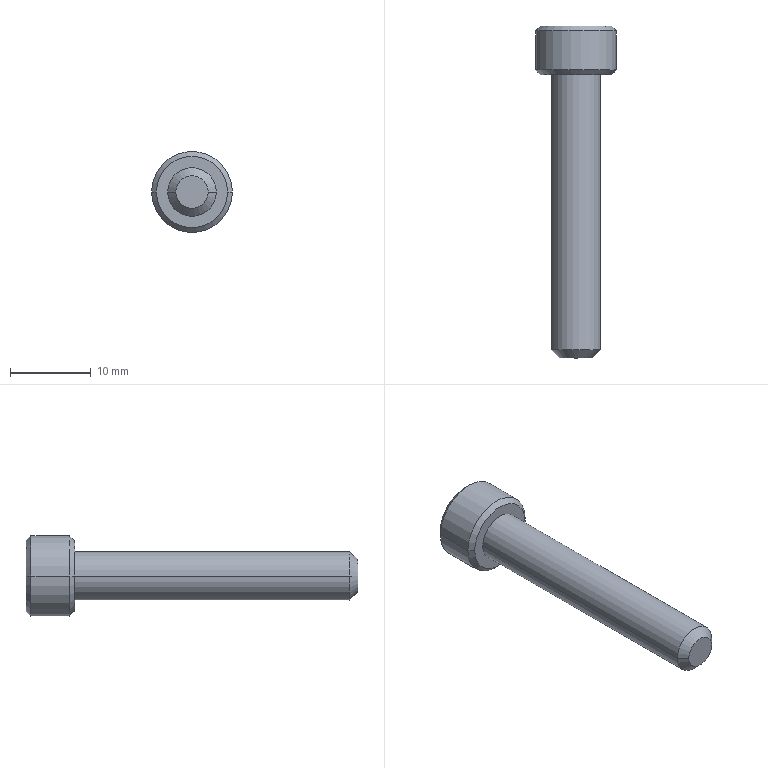Part | STEP file | BB62-M6-35L-3 | 1 solid | 27 faces | box 10 x 41 x 10 mm | volume 1364 mm3 | plane 15 | cone 8 | cylinder 4 | commonest cylinder face diameters 6 x2 10 x2
STEP:
#1=CARTESIAN_POINT('',(0.,1.349,0.));
#2=VERTEX_POINT('',#1);
#3=CARTESIAN_POINT('',(2.86,3.,0.));
#4=VERTEX_POINT('',#3);
#5=CARTESIAN_POINT('',(0.,1.349,0.));
#6=DIRECTION('',(0.866,0.5,0.));
#7=VECTOR('',#6,1000.);
#8=LINE('',#5,#7);
#9=EDGE_CURVE('',#2,#4,#8,.T.);
#10=ORIENTED_EDGE('',*,*,#9,.F.);
#11=CARTESIAN_POINT('',(-2.86,3.,0.));
#12=VERTEX_POINT('',#11);
#13=CARTESIAN_POINT('',(0.,1.349,0.));
#14=DIRECTION('',(-0.866,0.5,0.));
#15=VECTOR('',#14,1000.);
#16=LINE('',#13,#15);
#17=EDGE_CURVE('',#2,#12,#16,.T.);
#18=ORIENTED_EDGE('',*,*,#17,.T.);
#19=CARTESIAN_POINT('',(-2.477,3.,1.43));
#20=VERTEX_POINT('',#19);
#21=CARTESIAN_POINT('',(0.,3.,0.));
#22=DIRECTION('',(0.,-1.,0.));
#23=DIRECTION('',(-1.,0.,0.));
#24=AXIS2_PLACEMENT_3D('',#21,#22,#23);
#25=CIRCLE('',#24,2.86);
#26=EDGE_CURVE('',#20,#12,#25,.T.);
#27=ORIENTED_EDGE('',*,*,#26,.F.);
#28=CARTESIAN_POINT('',(0.,3.,2.86));
#29=VERTEX_POINT('',#28);
#30=CARTESIAN_POINT('',(0.,3.,0.));
#31=DIRECTION('',(0.,-1.,0.));
#32=DIRECTION('',(-1.,0.,0.));
#33=AXIS2_PLACEMENT_3D('',#30,#31,#32);
#34=CIRCLE('',#33,2.86);
#35=EDGE_CURVE('',#29,#20,#34,.T.);
#36=ORIENTED_EDGE('',*,*,#35,.F.);
#37=CARTESIAN_POINT('',(2.477,3.,1.43));
#38=VERTEX_POINT('',#37);
#39=CARTESIAN_POINT('',(0.,3.,0.));
#40=DIRECTION('',(0.,-1.,0.));
#41=DIRECTION('',(-1.,0.,0.));
#42=AXIS2_PLACEMENT_3D('',#39,#40,#41);
#43=CIRCLE('',#42,2.86);
#44=EDGE_CURVE('',#38,#29,#43,.T.);
#45=ORIENTED_EDGE('',*,*,#44,.F.);
#46=CARTESIAN_POINT('',(0.,3.,0.));
#47=DIRECTION('',(0.,-1.,0.));
#48=DIRECTION('',(-1.,0.,0.));
#49=AXIS2_PLACEMENT_3D('',#46,#47,#48);
#50=CIRCLE('',#49,2.86);
#51=EDGE_CURVE('',#4,#38,#50,.T.);
#52=ORIENTED_EDGE('',*,*,#51,.F.);
#53=EDGE_LOOP('',(#10,#18,#27,#36,#45,#52));
#54=FACE_OUTER_BOUND('',#53,.T.);
#55=CARTESIAN_POINT('',(0.,1001.349,0.));
#56=DIRECTION('',(0.,1.,0.));
#57=DIRECTION('',(1.,0.,0.));
#58=AXIS2_PLACEMENT_3D('',#55,#56,#57);
#59=CONICAL_SURFACE('',#58,1732.051,1.047);
#60=ADVANCED_FACE('',(#54),#59,.F.);
#61=CARTESIAN_POINT('',(2.,-35.,0.));
#62=VERTEX_POINT('',#61);
#63=CARTESIAN_POINT('',(-2.,-35.,0.));
#64=VERTEX_POINT('',#63);
#65=CARTESIAN_POINT('',(0.,-35.,0.));
#66=DIRECTION('',(0.,1.,0.));
#67=DIRECTION('',(1.,0.,0.));
#68=AXIS2_PLACEMENT_3D('',#65,#66,#67);
#69=CIRCLE('',#68,2.);
#70=EDGE_CURVE('',#62,#64,#69,.T.);
#71=ORIENTED_EDGE('',*,*,#70,.T.);
#72=CARTESIAN_POINT('',(-3.,-34.,0.));
#73=VERTEX_POINT('',#72);
#74=CARTESIAN_POINT('',(-2.,-35.,0.));
#75=DIRECTION('',(-0.7071,0.7071,0.));
#76=VECTOR('',#75,1000.);
#77=LINE('',#74,#76);
#78=EDGE_CURVE('',#64,#73,#77,.T.);
#79=ORIENTED_EDGE('',*,*,#78,.T.);
#80=CARTESIAN_POINT('',(3.,-34.,0.));
#81=VERTEX_POINT('',#80);
#82=CARTESIAN_POINT('',(0.,-34.,0.));
#83=DIRECTION('',(0.,-1.,0.));
#84=DIRECTION('',(-1.,0.,0.));
#85=AXIS2_PLACEMENT_3D('',#82,#83,#84);
#86=CIRCLE('',#85,3.);
#87=EDGE_CURVE('',#73,#81,#86,.T.);
#88=ORIENTED_EDGE('',*,*,#87,.T.);
#89=CARTESIAN_POINT('',(2.,-35.,0.));
#90=DIRECTION('',(0.7071,0.7071,0.));
#91=VECTOR('',#90,1000.);
#92=LINE('',#89,#91);
#93=EDGE_CURVE('',#62,#81,#92,.T.);
#94=ORIENTED_EDGE('',*,*,#93,.F.);
#95=EDGE_LOOP('',(#71,#79,#88,#94));
#96=FACE_OUTER_BOUND('',#95,.T.);
#97=CARTESIAN_POINT('',(0.,-35.,0.));
#98=DIRECTION('',(0.,1.,0.));
#99=DIRECTION('',(1.,0.,0.));
#100=AXIS2_PLACEMENT_3D('',#97,#98,#99);
#101=CONICAL_SURFACE('',#100,2.,0.7854);
#102=ADVANCED_FACE('',(#96),#101,.T.);
#103=ORIENTED_EDGE('',*,*,#87,.F.);
#104=CARTESIAN_POINT('',(-3.,0.,0.));
#105=VERTEX_POINT('',#104);
#106=CARTESIAN_POINT('',(-3.,-34.,0.));
#107=DIRECTION('',(0.,1.,0.));
#108=VECTOR('',#107,1000.);
#109=LINE('',#106,#108);
#110=EDGE_CURVE('',#73,#105,#109,.T.);
#111=ORIENTED_EDGE('',*,*,#110,.T.);
#112=CARTESIAN_POINT('',(3.,0.,0.));
#113=VERTEX_POINT('',#112);
#114=CARTESIAN_POINT('',(0.,0.,0.));
#115=DIRECTION('',(0.,-1.,0.));
#116=DIRECTION('',(-1.,0.,0.));
#117=AXIS2_PLACEMENT_3D('',#114,#115,#116);
#118=CIRCLE('',#117,3.);
#119=EDGE_CURVE('',#105,#113,#118,.T.);
#120=ORIENTED_EDGE('',*,*,#119,.T.);
#121=CARTESIAN_POINT('',(3.,-34.,0.));
#122=DIRECTION('',(0.,1.,0.));
#123=VECTOR('',#122,1000.);
#124=LINE('',#121,#123);
#125=EDGE_CURVE('',#81,#113,#124,.T.);
#126=ORIENTED_EDGE('',*,*,#125,.F.);
#127=EDGE_LOOP('',(#103,#111,#120,#126));
#128=FACE_OUTER_BOUND('',#127,.T.);
#129=CARTESIAN_POINT('',(0.,-34.,0.));
#130=DIRECTION('',(0.,1.,0.));
#131=DIRECTION('',(1.,0.,0.));
#132=AXIS2_PLACEMENT_3D('',#129,#130,#131);
#133=CYLINDRICAL_SURFACE('',#132,3.);
#134=ADVANCED_FACE('',(#128),#133,.T.);
#135=CARTESIAN_POINT('',(-4.4,6.,0.));
#136=VERTEX_POINT('',#135);
#137=CARTESIAN_POINT('',(4.4,6.,0.));
#138=VERTEX_POINT('',#137);
#139=CARTESIAN_POINT('',(0.,6.,0.));
#140=DIRECTION('',(0.,-1.,0.));
#141=DIRECTION('',(-1.,0.,0.));
#142=AXIS2_PLACEMENT_3D('',#139,#140,#141);
#143=CIRCLE('',#142,4.4);
#144=EDGE_CURVE('',#136,#138,#143,.T.);
#145=ORIENTED_EDGE('',*,*,#144,.T.);
#146=CARTESIAN_POINT('',(5.,5.4,0.));
#147=VERTEX_POINT('',#146);
#148=CARTESIAN_POINT('',(5.,5.4,0.));
#149=DIRECTION('',(0.7071,-0.7071,0.));
#150=VECTOR('',#149,1000.);
#151=LINE('',#148,#150);
#152=EDGE_CURVE('',#138,#147,#151,.T.);
#153=ORIENTED_EDGE('',*,*,#152,.T.);
#154=CARTESIAN_POINT('',(-5.,5.4,0.));
#155=VERTEX_POINT('',#154);
#156=CARTESIAN_POINT('',(0.,5.4,0.));
#157=DIRECTION('',(0.,-1.,0.));
#158=DIRECTION('',(-1.,0.,0.));
#159=AXIS2_PLACEMENT_3D('',#156,#157,#158);
#160=CIRCLE('',#159,5.);
#161=EDGE_CURVE('',#155,#147,#160,.T.);
#162=ORIENTED_EDGE('',*,*,#161,.F.);
#163=CARTESIAN_POINT('',(-5.,5.4,0.));
#164=DIRECTION('',(-0.7071,-0.7071,0.));
#165=VECTOR('',#164,1000.);
#166=LINE('',#163,#165);
#167=EDGE_CURVE('',#136,#155,#166,.T.);
#168=ORIENTED_EDGE('',*,*,#167,.F.);
#169=EDGE_LOOP('',(#145,#153,#162,#168));
#170=FACE_OUTER_BOUND('',#169,.T.);
#171=CARTESIAN_POINT('',(0.,5.4,0.));
#172=DIRECTION('',(0.,-1.,0.));
#173=DIRECTION('',(-1.,0.,0.));
#174=AXIS2_PLACEMENT_3D('',#171,#172,#173);
#175=CONICAL_SURFACE('',#174,5.,0.7854);
#176=ADVANCED_FACE('',(#170),#175,.T.);
#177=ORIENTED_EDGE('',*,*,#161,.T.);
#178=CARTESIAN_POINT('',(5.,0.6,0.));
#179=VERTEX_POINT('',#178);
#180=CARTESIAN_POINT('',(5.,1.62,0.));
#181=DIRECTION('',(0.,-1.,0.));
#182=VECTOR('',#181,1000.);
#183=LINE('',#180,#182);
#184=EDGE_CURVE('',#147,#179,#183,.T.);
#185=ORIENTED_EDGE('',*,*,#184,.T.);
#186=CARTESIAN_POINT('',(-5.,0.6,0.));
#187=VERTEX_POINT('',#186);
#188=CARTESIAN_POINT('',(0.,0.6,0.));
#189=DIRECTION('',(0.,-1.,0.));
#190=DIRECTION('',(-1.,0.,0.));
#191=AXIS2_PLACEMENT_3D('',#188,#189,#190);
#192=CIRCLE('',#191,5.);
#193=EDGE_CURVE('',#187,#179,#192,.T.);
#194=ORIENTED_EDGE('',*,*,#193,.F.);
#195=CARTESIAN_POINT('',(-5.,1.62,0.));
#196=DIRECTION('',(0.,-1.,0.));
#197=VECTOR('',#196,1000.);
#198=LINE('',#195,#197);
#199=EDGE_CURVE('',#155,#187,#198,.T.);
#200=ORIENTED_EDGE('',*,*,#199,.F.);
#201=EDGE_LOOP('',(#177,#185,#194,#200));
#202=FACE_OUTER_BOUND('',#201,.T.);
#203=CARTESIAN_POINT('',(0.,1.62,0.));
#204=DIRECTION('',(0.,-1.,0.));
#205=DIRECTION('',(-1.,0.,0.));
#206=AXIS2_PLACEMENT_3D('',#203,#204,#205);
#207=CYLINDRICAL_SURFACE('',#206,5.);
#208=ADVANCED_FACE('',(#202),#207,.T.);
#209=CARTESIAN_POINT('',(-4.4,0.,0.));
#210=VERTEX_POINT('',#209);
#211=CARTESIAN_POINT('',(4.4,0.,0.));
#212=VERTEX_POINT('',#211);
#213=CARTESIAN_POINT('',(0.,0.,0.));
#214=DIRECTION('',(0.,-1.,0.));
#215=DIRECTION('',(-1.,0.,0.));
#216=AXIS2_PLACEMENT_3D('',#213,#214,#215);
#217=CIRCLE('',#216,4.4);
#218=EDGE_CURVE('',#210,#212,#217,.T.);
#219=ORIENTED_EDGE('',*,*,#218,.F.);
#220=CARTESIAN_POINT('',(-4.4,0.,0.));
#221=DIRECTION('',(-0.7071,0.7071,0.));
#222=VECTOR('',#221,1000.);
#223=LINE('',#220,#222);
#224=EDGE_CURVE('',#210,#187,#223,.T.);
#225=ORIENTED_EDGE('',*,*,#224,.T.);
#226=ORIENTED_EDGE('',*,*,#193,.T.);
#227=CARTESIAN_POINT('',(4.4,0.,0.));
#228=DIRECTION('',(0.7071,0.7071,0.));
#229=VECTOR('',#228,1000.);
#230=LINE('',#227,#229);
#231=EDGE_CURVE('',#212,#179,#230,.T.);
#232=ORIENTED_EDGE('',*,*,#231,.F.);
#233=EDGE_LOOP('',(#219,#225,#226,#232));
#234=FACE_OUTER_BOUND('',#233,.T.);
#235=CARTESIAN_POINT('',(0.,0.,0.));
#236=DIRECTION('',(0.,1.,0.));
#237=DIRECTION('',(1.,0.,0.));
#238=AXIS2_PLACEMENT_3D('',#235,#236,#237);
#239=CONICAL_SURFACE('',#238,4.4,0.7854);
#240=ADVANCED_FACE('',(#234),#239,.T.);
#241=ORIENTED_EDGE('',*,*,#144,.F.);
#242=CARTESIAN_POINT('',(0.,6.,0.));
#243=DIRECTION('',(0.,-1.,0.));
#244=DIRECTION('',(-1.,0.,0.));
#245=AXIS2_PLACEMENT_3D('',#242,#243,#244);
#246=CIRCLE('',#245,4.4);
#247=EDGE_CURVE('',#138,#136,#246,.T.);
#248=ORIENTED_EDGE('',*,*,#247,.F.);
#249=EDGE_LOOP('',(#241,#248));
#250=FACE_OUTER_BOUND('',#249,.T.);
#251=CARTESIAN_POINT('',(0.,6.,-2.86));
#252=VERTEX_POINT('',#251);
#253=CARTESIAN_POINT('',(-2.477,6.,-1.43));
#254=VERTEX_POINT('',#253);
#255=CARTESIAN_POINT('',(0.,6.,-2.86));
#256=DIRECTION('',(-0.866,0.,0.5));
#257=VECTOR('',#256,1000.);
#258=LINE('',#255,#257);
#259=EDGE_CURVE('',#252,#254,#258,.T.);
#260=ORIENTED_EDGE('',*,*,#259,.F.);
#261=CARTESIAN_POINT('',(2.477,6.,-1.43));
#262=VERTEX_POINT('',#261);
#263=CARTESIAN_POINT('',(2.477,6.,-1.43));
#264=DIRECTION('',(-0.866,0.,-0.5));
#265=VECTOR('',#264,1000.);
#266=LINE('',#263,#265);
#267=EDGE_CURVE('',#262,#252,#266,.T.);
#268=ORIENTED_EDGE('',*,*,#267,.F.);
#269=CARTESIAN_POINT('',(2.477,6.,1.43));
#270=VERTEX_POINT('',#269);
#271=CARTESIAN_POINT('',(2.477,6.,1.43));
#272=DIRECTION('',(0.,0.,-1.));
#273=VECTOR('',#272,1000.);
#274=LINE('',#271,#273);
#275=EDGE_CURVE('',#270,#262,#274,.T.);
#276=ORIENTED_EDGE('',*,*,#275,.F.);
#277=CARTESIAN_POINT('',(0.,6.,2.86));
#278=VERTEX_POINT('',#277);
#279=CARTESIAN_POINT('',(0.,6.,2.86));
#280=DIRECTION('',(0.866,0.,-0.5));
#281=VECTOR('',#280,1000.);
#282=LINE('',#279,#281);
#283=EDGE_CURVE('',#278,#270,#282,.T.);
#284=ORIENTED_EDGE('',*,*,#283,.F.);
#285=CARTESIAN_POINT('',(-2.477,6.,1.43));
#286=VERTEX_POINT('',#285);
#287=CARTESIAN_POINT('',(-2.477,6.,1.43));
#288=DIRECTION('',(0.866,0.,0.5));
#289=VECTOR('',#288,1000.);
#290=LINE('',#287,#289);
#291=EDGE_CURVE('',#286,#278,#290,.T.);
#292=ORIENTED_EDGE('',*,*,#291,.F.);
#293=CARTESIAN_POINT('',(-2.477,6.,-1.43));
#294=DIRECTION('',(0.,0.,1.));
#295=VECTOR('',#294,1000.);
#296=LINE('',#293,#295);
#297=EDGE_CURVE('',#254,#286,#296,.T.);
#298=ORIENTED_EDGE('',*,*,#297,.F.);
#299=EDGE_LOOP('',(#260,#268,#276,#284,#292,#298));
#300=FACE_BOUND('',#299,.T.);
#301=CARTESIAN_POINT('',(4.4,6.,0.));
#302=DIRECTION('',(0.,1.,0.));
#303=DIRECTION('',(1.,0.,0.));
#304=AXIS2_PLACEMENT_3D('',#301,#302,#303);
#305=PLANE('',#304);
#306=ADVANCED_FACE('',(#250,#300),#305,.T.);
#307=CARTESIAN_POINT('',(0.,0.,0.));
#308=DIRECTION('',(0.,-1.,0.));
#309=DIRECTION('',(-1.,0.,0.));
#310=AXIS2_PLACEMENT_3D('',#307,#308,#309);
#311=CIRCLE('',#310,3.);
#312=EDGE_CURVE('',#113,#105,#311,.T.);
#313=ORIENTED_EDGE('',*,*,#312,.F.);
#314=ORIENTED_EDGE('',*,*,#119,.F.);
#315=EDGE_LOOP('',(#313,#314));
#316=FACE_BOUND('',#315,.T.);
#317=CARTESIAN_POINT('',(0.,0.,0.));
#318=DIRECTION('',(0.,-1.,0.));
#319=DIRECTION('',(-1.,0.,0.));
#320=AXIS2_PLACEMENT_3D('',#317,#318,#319);
#321=CIRCLE('',#320,4.4);
#322=EDGE_CURVE('',#212,#210,#321,.T.);
#323=ORIENTED_EDGE('',*,*,#322,.T.);
#324=ORIENTED_EDGE('',*,*,#218,.T.);
#325=EDGE_LOOP('',(#323,#324));
#326=FACE_OUTER_BOUND('',#325,.T.);
#327=CARTESIAN_POINT('',(0.,0.,0.));
#328=DIRECTION('',(0.,-1.,0.));
#329=DIRECTION('',(-1.,0.,0.));
#330=AXIS2_PLACEMENT_3D('',#327,#328,#329);
#331=PLANE('',#330);
#332=ADVANCED_FACE('',(#316,#326),#331,.T.);
#333=ORIENTED_EDGE('',*,*,#224,.F.);
#334=ORIENTED_EDGE('',*,*,#322,.F.);
#335=ORIENTED_EDGE('',*,*,#231,.T.);
#336=CARTESIAN_POINT('',(0.,0.6,0.));
#337=DIRECTION('',(0.,-1.,0.));
#338=DIRECTION('',(-1.,0.,0.));
#339=AXIS2_PLACEMENT_3D('',#336,#337,#338);
#340=CIRCLE('',#339,5.);
#341=EDGE_CURVE('',#179,#187,#340,.T.);
#342=ORIENTED_EDGE('',*,*,#341,.T.);
#343=EDGE_LOOP('',(#333,#334,#335,#342));
#344=FACE_OUTER_BOUND('',#343,.T.);
#345=CARTESIAN_POINT('',(0.,0.,0.));
#346=DIRECTION('',(0.,1.,0.));
#347=DIRECTION('',(1.,0.,0.));
#348=AXIS2_PLACEMENT_3D('',#345,#346,#347);
#349=CONICAL_SURFACE('',#348,4.4,0.7854);
#350=ADVANCED_FACE('',(#344),#349,.T.);
#351=ORIENTED_EDGE('',*,*,#184,.F.);
#352=CARTESIAN_POINT('',(0.,5.4,0.));
#353=DIRECTION('',(0.,-1.,0.));
#354=DIRECTION('',(-1.,0.,0.));
#355=AXIS2_PLACEMENT_3D('',#352,#353,#354);
#356=CIRCLE('',#355,5.);
#357=EDGE_CURVE('',#147,#155,#356,.T.);
#358=ORIENTED_EDGE('',*,*,#357,.T.);
#359=ORIENTED_EDGE('',*,*,#199,.T.);
#360=ORIENTED_EDGE('',*,*,#341,.F.);
#361=EDGE_LOOP('',(#351,#358,#359,#360));
#362=FACE_OUTER_BOUND('',#361,.T.);
#363=CARTESIAN_POINT('',(0.,1.62,0.));
#364=DIRECTION('',(0.,-1.,0.));
#365=DIRECTION('',(-1.,0.,0.));
#366=AXIS2_PLACEMENT_3D('',#363,#364,#365);
#367=CYLINDRICAL_SURFACE('',#366,5.);
#368=ADVANCED_FACE('',(#362),#367,.T.);
#369=ORIENTED_EDGE('',*,*,#152,.F.);
#370=ORIENTED_EDGE('',*,*,#247,.T.);
#371=ORIENTED_EDGE('',*,*,#167,.T.);
#372=ORIENTED_EDGE('',*,*,#357,.F.);
#373=EDGE_LOOP('',(#369,#370,#371,#372));
#374=FACE_OUTER_BOUND('',#373,.T.);
#375=CARTESIAN_POINT('',(0.,5.4,0.));
#376=DIRECTION('',(0.,-1.,0.));
#377=DIRECTION('',(-1.,0.,0.));
#378=AXIS2_PLACEMENT_3D('',#375,#376,#377);
#379=CONICAL_SURFACE('',#378,5.,0.7854);
#380=ADVANCED_FACE('',(#374),#379,.T.);
#381=ORIENTED_EDGE('',*,*,#110,.F.);
#382=CARTESIAN_POINT('',(0.,-34.,0.));
#383=DIRECTION('',(0.,-1.,0.));
#384=DIRECTION('',(-1.,0.,0.));
#385=AXIS2_PLACEMENT_3D('',#382,#383,#384);
#386=CIRCLE('',#385,3.);
#387=EDGE_CURVE('',#81,#73,#386,.T.);
#388=ORIENTED_EDGE('',*,*,#387,.F.);
#389=ORIENTED_EDGE('',*,*,#125,.T.);
#390=ORIENTED_EDGE('',*,*,#312,.T.);
#391=EDGE_LOOP('',(#381,#388,#389,#390));
#392=FACE_OUTER_BOUND('',#391,.T.);
#393=CARTESIAN_POINT('',(0.,-34.,0.));
#394=DIRECTION('',(0.,1.,0.));
#395=DIRECTION('',(1.,0.,0.));
#396=AXIS2_PLACEMENT_3D('',#393,#394,#395);
#397=CYLINDRICAL_SURFACE('',#396,3.);
#398=ADVANCED_FACE('',(#392),#397,.T.);
#399=ORIENTED_EDGE('',*,*,#70,.F.);
#400=CARTESIAN_POINT('',(0.,-35.,0.));
#401=DIRECTION('',(0.,1.,0.));
#402=DIRECTION('',(1.,0.,0.));
#403=AXIS2_PLACEMENT_3D('',#400,#401,#402);
#404=CIRCLE('',#403,2.);
#405=EDGE_CURVE('',#64,#62,#404,.T.);
#406=ORIENTED_EDGE('',*,*,#405,.F.);
#407=EDGE_LOOP('',(#399,#406));
#408=FACE_OUTER_BOUND('',#407,.T.);
#409=CARTESIAN_POINT('',(0.,-35.,0.));
#410=DIRECTION('',(0.,-1.,0.));
#411=DIRECTION('',(-1.,0.,0.));
#412=AXIS2_PLACEMENT_3D('',#409,#410,#411);
#413=PLANE('',#412);
#414=ADVANCED_FACE('',(#408),#413,.T.);
#415=ORIENTED_EDGE('',*,*,#78,.F.);
#416=ORIENTED_EDGE('',*,*,#405,.T.);
#417=ORIENTED_EDGE('',*,*,#93,.T.);
#418=ORIENTED_EDGE('',*,*,#387,.T.);
#419=EDGE_LOOP('',(#415,#416,#417,#418));
#420=FACE_OUTER_BOUND('',#419,.T.);
#421=CARTESIAN_POINT('',(0.,-35.,0.));
#422=DIRECTION('',(0.,1.,0.));
#423=DIRECTION('',(1.,0.,0.));
#424=AXIS2_PLACEMENT_3D('',#421,#422,#423);
#425=CONICAL_SURFACE('',#424,2.,0.7854);
#426=ADVANCED_FACE('',(#420),#425,.T.);
#427=CARTESIAN_POINT('',(2.477,3.,-1.43));
#428=VERTEX_POINT('',#427);
#429=CARTESIAN_POINT('',(0.,3.,-2.86));
#430=VERTEX_POINT('',#429);
#431=CARTESIAN_POINT('',(2.477,3.,-1.43));
#432=DIRECTION('',(-0.866,0.,-0.5));
#433=VECTOR('',#432,1000.);
#434=LINE('',#431,#433);
#435=EDGE_CURVE('',#428,#430,#434,.T.);
#436=ORIENTED_EDGE('',*,*,#435,.F.);
#437=CARTESIAN_POINT('',(2.477,6.,-1.43));
#438=DIRECTION('',(0.,-1.,0.));
#439=VECTOR('',#438,1000.);
#440=LINE('',#437,#439);
#441=EDGE_CURVE('',#262,#428,#440,.T.);
#442=ORIENTED_EDGE('',*,*,#441,.F.);
#443=ORIENTED_EDGE('',*,*,#267,.T.);
#444=CARTESIAN_POINT('',(0.,6.,-2.86));
#445=DIRECTION('',(0.,-1.,0.));
#446=VECTOR('',#445,1000.);
#447=LINE('',#444,#446);
#448=EDGE_CURVE('',#252,#430,#447,.T.);
#449=ORIENTED_EDGE('',*,*,#448,.T.);
#450=EDGE_LOOP('',(#436,#442,#443,#449));
#451=FACE_OUTER_BOUND('',#450,.T.);
#452=CARTESIAN_POINT('',(2.477,6.,-1.43));
#453=DIRECTION('',(-0.5,0.,0.866));
#454=DIRECTION('',(0.866,0.,0.5));
#455=AXIS2_PLACEMENT_3D('',#452,#453,#454);
#456=PLANE('',#455);
#457=ADVANCED_FACE('',(#451),#456,.T.);
#458=CARTESIAN_POINT('',(-2.477,3.,-1.43));
#459=VERTEX_POINT('',#458);
#460=CARTESIAN_POINT('',(0.,3.,-2.86));
#461=DIRECTION('',(-0.866,0.,0.5));
#462=VECTOR('',#461,1000.);
#463=LINE('',#460,#462);
#464=EDGE_CURVE('',#430,#459,#463,.T.);
#465=ORIENTED_EDGE('',*,*,#464,.F.);
#466=ORIENTED_EDGE('',*,*,#448,.F.);
#467=ORIENTED_EDGE('',*,*,#259,.T.);
#468=CARTESIAN_POINT('',(-2.477,6.,-1.43));
#469=DIRECTION('',(0.,-1.,0.));
#470=VECTOR('',#469,1000.);
#471=LINE('',#468,#470);
#472=EDGE_CURVE('',#254,#459,#471,.T.);
#473=ORIENTED_EDGE('',*,*,#472,.T.);
#474=EDGE_LOOP('',(#465,#466,#467,#473));
#475=FACE_OUTER_BOUND('',#474,.T.);
#476=CARTESIAN_POINT('',(0.,6.,-2.86));
#477=DIRECTION('',(0.5,0.,0.866));
#478=DIRECTION('',(0.866,0.,-0.5));
#479=AXIS2_PLACEMENT_3D('',#476,#477,#478);
#480=PLANE('',#479);
#481=ADVANCED_FACE('',(#475),#480,.T.);
#482=CARTESIAN_POINT('',(-2.477,3.,-1.43));
#483=DIRECTION('',(0.,0.,1.));
#484=VECTOR('',#483,1000.);
#485=LINE('',#482,#484);
#486=EDGE_CURVE('',#459,#20,#485,.T.);
#487=ORIENTED_EDGE('',*,*,#486,.F.);
#488=ORIENTED_EDGE('',*,*,#472,.F.);
#489=ORIENTED_EDGE('',*,*,#297,.T.);
#490=CARTESIAN_POINT('',(-2.477,6.,1.43));
#491=DIRECTION('',(0.,-1.,0.));
#492=VECTOR('',#491,1000.);
#493=LINE('',#490,#492);
#494=EDGE_CURVE('',#286,#20,#493,.T.);
#495=ORIENTED_EDGE('',*,*,#494,.T.);
#496=EDGE_LOOP('',(#487,#488,#489,#495));
#497=FACE_OUTER_BOUND('',#496,.T.);
#498=CARTESIAN_POINT('',(-2.477,6.,-1.43));
#499=DIRECTION('',(1.,0.,0.));
#500=DIRECTION('',(0.,0.,-1.));
#501=AXIS2_PLACEMENT_3D('',#498,#499,#500);
#502=PLANE('',#501);
#503=ADVANCED_FACE('',(#497),#502,.T.);
#504=CARTESIAN_POINT('',(-2.477,3.,1.43));
#505=DIRECTION('',(0.866,0.,0.5));
#506=VECTOR('',#505,1000.);
#507=LINE('',#504,#506);
#508=EDGE_CURVE('',#20,#29,#507,.T.);
#509=ORIENTED_EDGE('',*,*,#508,.F.);
#510=ORIENTED_EDGE('',*,*,#494,.F.);
#511=ORIENTED_EDGE('',*,*,#291,.T.);
#512=CARTESIAN_POINT('',(0.,6.,2.86));
#513=DIRECTION('',(0.,-1.,0.));
#514=VECTOR('',#513,1000.);
#515=LINE('',#512,#514);
#516=EDGE_CURVE('',#278,#29,#515,.T.);
#517=ORIENTED_EDGE('',*,*,#516,.T.);
#518=EDGE_LOOP('',(#509,#510,#511,#517));
#519=FACE_OUTER_BOUND('',#518,.T.);
#520=CARTESIAN_POINT('',(-2.477,6.,1.43));
#521=DIRECTION('',(0.5,0.,-0.866));
#522=DIRECTION('',(-0.866,0.,-0.5));
#523=AXIS2_PLACEMENT_3D('',#520,#521,#522);
#524=PLANE('',#523);
#525=ADVANCED_FACE('',(#519),#524,.T.);
#526=CARTESIAN_POINT('',(0.,3.,2.86));
#527=DIRECTION('',(0.866,0.,-0.5));
#528=VECTOR('',#527,1000.);
#529=LINE('',#526,#528);
#530=EDGE_CURVE('',#29,#38,#529,.T.);
#531=ORIENTED_EDGE('',*,*,#530,.F.);
#532=ORIENTED_EDGE('',*,*,#516,.F.);
#533=ORIENTED_EDGE('',*,*,#283,.T.);
#534=CARTESIAN_POINT('',(2.477,6.,1.43));
#535=DIRECTION('',(0.,-1.,0.));
#536=VECTOR('',#535,1000.);
#537=LINE('',#534,#536);
#538=EDGE_CURVE('',#270,#38,#537,.T.);
#539=ORIENTED_EDGE('',*,*,#538,.T.);
#540=EDGE_LOOP('',(#531,#532,#533,#539));
#541=FACE_OUTER_BOUND('',#540,.T.);
#542=CARTESIAN_POINT('',(0.,6.,2.86));
#543=DIRECTION('',(-0.5,0.,-0.866));
#544=DIRECTION('',(-0.866,0.,0.5));
#545=AXIS2_PLACEMENT_3D('',#542,#543,#544);
#546=PLANE('',#545);
#547=ADVANCED_FACE('',(#541),#546,.T.);
#548=CARTESIAN_POINT('',(2.477,3.,1.43));
#549=DIRECTION('',(0.,0.,-1.));
#550=VECTOR('',#549,1000.);
#551=LINE('',#548,#550);
#552=EDGE_CURVE('',#38,#428,#551,.T.);
#553=ORIENTED_EDGE('',*,*,#552,.F.);
#554=ORIENTED_EDGE('',*,*,#538,.F.);
#555=ORIENTED_EDGE('',*,*,#275,.T.);
#556=ORIENTED_EDGE('',*,*,#441,.T.);
#557=EDGE_LOOP('',(#553,#554,#555,#556));
#558=FACE_OUTER_BOUND('',#557,.T.);
#559=CARTESIAN_POINT('',(2.477,6.,1.43));
#560=DIRECTION('',(-1.,0.,0.));
#561=DIRECTION('',(0.,0.,1.));
#562=AXIS2_PLACEMENT_3D('',#559,#560,#561);
#563=PLANE('',#562);
#564=ADVANCED_FACE('',(#558),#563,.T.);
#565=ORIENTED_EDGE('',*,*,#435,.T.);
#566=CARTESIAN_POINT('',(0.,3.,0.));
#567=DIRECTION('',(0.,-1.,0.));
#568=DIRECTION('',(-1.,0.,0.));
#569=AXIS2_PLACEMENT_3D('',#566,#567,#568);
#570=CIRCLE('',#569,2.86);
#571=EDGE_CURVE('',#430,#428,#570,.T.);
#572=ORIENTED_EDGE('',*,*,#571,.T.);
#573=EDGE_LOOP('',(#565,#572));
#574=FACE_OUTER_BOUND('',#573,.T.);
#575=CARTESIAN_POINT('',(0.,3.,0.));
#576=DIRECTION('',(0.,1.,0.));
#577=DIRECTION('',(1.,0.,0.));
#578=AXIS2_PLACEMENT_3D('',#575,#576,#577);
#579=PLANE('',#578);
#580=ADVANCED_FACE('',(#574),#579,.F.);
#581=ORIENTED_EDGE('',*,*,#552,.T.);
#582=CARTESIAN_POINT('',(0.,3.,0.));
#583=DIRECTION('',(0.,-1.,0.));
#584=DIRECTION('',(-1.,0.,0.));
#585=AXIS2_PLACEMENT_3D('',#582,#583,#584);
#586=CIRCLE('',#585,2.86);
#587=EDGE_CURVE('',#428,#4,#586,.T.);
#588=ORIENTED_EDGE('',*,*,#587,.T.);
#589=ORIENTED_EDGE('',*,*,#51,.T.);
#590=EDGE_LOOP('',(#581,#588,#589));
#591=FACE_OUTER_BOUND('',#590,.T.);
#592=CARTESIAN_POINT('',(0.,3.,0.));
#593=DIRECTION('',(0.,1.,0.));
#594=DIRECTION('',(1.,0.,0.));
#595=AXIS2_PLACEMENT_3D('',#592,#593,#594);
#596=PLANE('',#595);
#597=ADVANCED_FACE('',(#591),#596,.F.);
#598=ORIENTED_EDGE('',*,*,#530,.T.);
#599=ORIENTED_EDGE('',*,*,#44,.T.);
#600=EDGE_LOOP('',(#598,#599));
#601=FACE_OUTER_BOUND('',#600,.T.);
#602=CARTESIAN_POINT('',(0.,3.,0.));
#603=DIRECTION('',(0.,1.,0.));
#604=DIRECTION('',(1.,0.,0.));
#605=AXIS2_PLACEMENT_3D('',#602,#603,#604);
#606=PLANE('',#605);
#607=ADVANCED_FACE('',(#601),#606,.F.);
#608=ORIENTED_EDGE('',*,*,#508,.T.);
#609=ORIENTED_EDGE('',*,*,#35,.T.);
#610=EDGE_LOOP('',(#608,#609));
#611=FACE_OUTER_BOUND('',#610,.T.);
#612=CARTESIAN_POINT('',(0.,3.,0.));
#613=DIRECTION('',(0.,1.,0.));
#614=DIRECTION('',(1.,0.,0.));
#615=AXIS2_PLACEMENT_3D('',#612,#613,#614);
#616=PLANE('',#615);
#617=ADVANCED_FACE('',(#611),#616,.F.);
#618=ORIENTED_EDGE('',*,*,#486,.T.);
#619=ORIENTED_EDGE('',*,*,#26,.T.);
#620=CARTESIAN_POINT('',(0.,3.,0.));
#621=DIRECTION('',(0.,-1.,0.));
#622=DIRECTION('',(-1.,0.,0.));
#623=AXIS2_PLACEMENT_3D('',#620,#621,#622);
#624=CIRCLE('',#623,2.86);
#625=EDGE_CURVE('',#12,#459,#624,.T.);
#626=ORIENTED_EDGE('',*,*,#625,.T.);
#627=EDGE_LOOP('',(#618,#619,#626));
#628=FACE_OUTER_BOUND('',#627,.T.);
#629=CARTESIAN_POINT('',(0.,3.,0.));
#630=DIRECTION('',(0.,1.,0.));
#631=DIRECTION('',(1.,0.,0.));
#632=AXIS2_PLACEMENT_3D('',#629,#630,#631);
#633=PLANE('',#632);
#634=ADVANCED_FACE('',(#628),#633,.F.);
#635=ORIENTED_EDGE('',*,*,#464,.T.);
#636=CARTESIAN_POINT('',(0.,3.,0.));
#637=DIRECTION('',(0.,-1.,0.));
#638=DIRECTION('',(-1.,0.,0.));
#639=AXIS2_PLACEMENT_3D('',#636,#637,#638);
#640=CIRCLE('',#639,2.86);
#641=EDGE_CURVE('',#459,#430,#640,.T.);
#642=ORIENTED_EDGE('',*,*,#641,.T.);
#643=EDGE_LOOP('',(#635,#642));
#644=FACE_OUTER_BOUND('',#643,.T.);
#645=CARTESIAN_POINT('',(0.,3.,0.));
#646=DIRECTION('',(0.,1.,0.));
#647=DIRECTION('',(1.,0.,0.));
#648=AXIS2_PLACEMENT_3D('',#645,#646,#647);
#649=PLANE('',#648);
#650=ADVANCED_FACE('',(#644),#649,.F.);
#651=ORIENTED_EDGE('',*,*,#17,.F.);
#652=ORIENTED_EDGE('',*,*,#9,.T.);
#653=ORIENTED_EDGE('',*,*,#587,.F.);
#654=ORIENTED_EDGE('',*,*,#571,.F.);
#655=ORIENTED_EDGE('',*,*,#641,.F.);
#656=ORIENTED_EDGE('',*,*,#625,.F.);
#657=EDGE_LOOP('',(#651,#652,#653,#654,#655,#656));
#658=FACE_OUTER_BOUND('',#657,.T.);
#659=CARTESIAN_POINT('',(0.,1001.349,0.));
#660=DIRECTION('',(0.,1.,0.));
#661=DIRECTION('',(1.,0.,0.));
#662=AXIS2_PLACEMENT_3D('',#659,#660,#661);
#663=CONICAL_SURFACE('',#662,1732.051,1.047);
#664=ADVANCED_FACE('',(#658),#663,.F.);
#665=CLOSED_SHELL('',(#60,#102,#134,#176,#208,#240,#306,#332,#350,#368,#380,#398,#414,#426,#457,#481,#503,#525,#547,#564,#580,#597,#607,#617,#634,#650,#664));
#666=MANIFOLD_SOLID_BREP('',#665);
#667=CARTESIAN_POINT('',(0.,0.,0.));
#668=DIRECTION('',(0.,0.,1.));
#669=DIRECTION('',(1.,0.,0.));
#670=AXIS2_PLACEMENT_3D('',#667,#668,#669);
#671=(LENGTH_UNIT()NAMED_UNIT(*)SI_UNIT(.MILLI.,.METRE.));
#672=UNCERTAINTY_MEASURE_WITH_UNIT(LENGTH_MEASURE(0.00001),#671,'','');
#673=(NAMED_UNIT(*)PLANE_ANGLE_UNIT()SI_UNIT($,.RADIAN.));
#674=(NAMED_UNIT(*)SI_UNIT($,.STERADIAN.)SOLID_ANGLE_UNIT());
#675=(GEOMETRIC_REPRESENTATION_CONTEXT(3)GLOBAL_UNCERTAINTY_ASSIGNED_CONTEXT((#672))GLOBAL_UNIT_ASSIGNED_CONTEXT((#671,#673,#674))REPRESENTATION_CONTEXT('',''));
#676=ADVANCED_BREP_SHAPE_REPRESENTATION('',(#666,#670),#675);